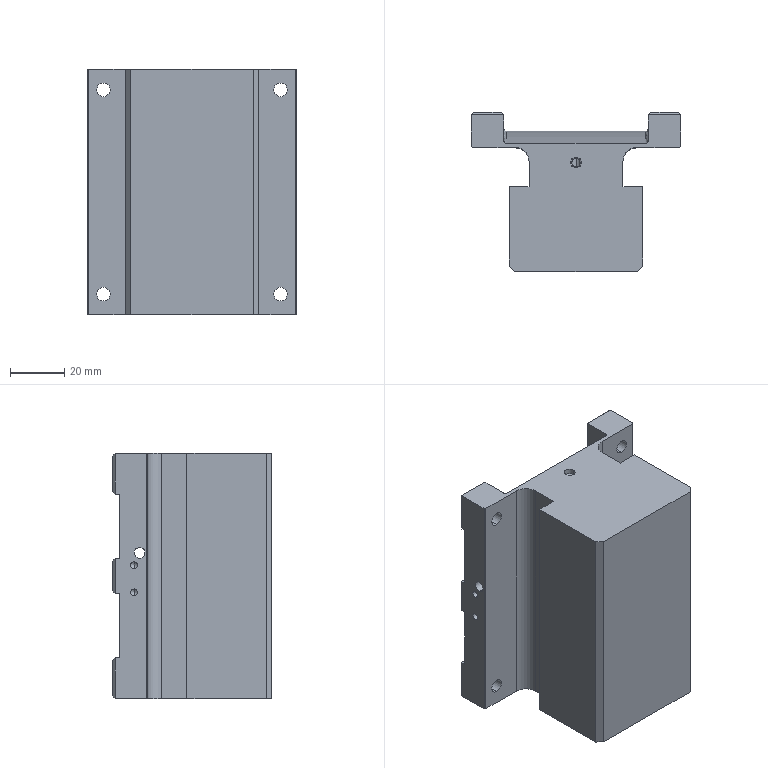Part | NX | features BREP 1 | 1 solid | 125 faces | box 77 x 58.5 x 90 mm | volume 226151 mm3 | plane 62 | cylinder 39 | cone 22 | torus 2 | commonest cylinder face diameters 2.5 x16 5 x12 3 x4 4 x4 10 x2 454.5 x1